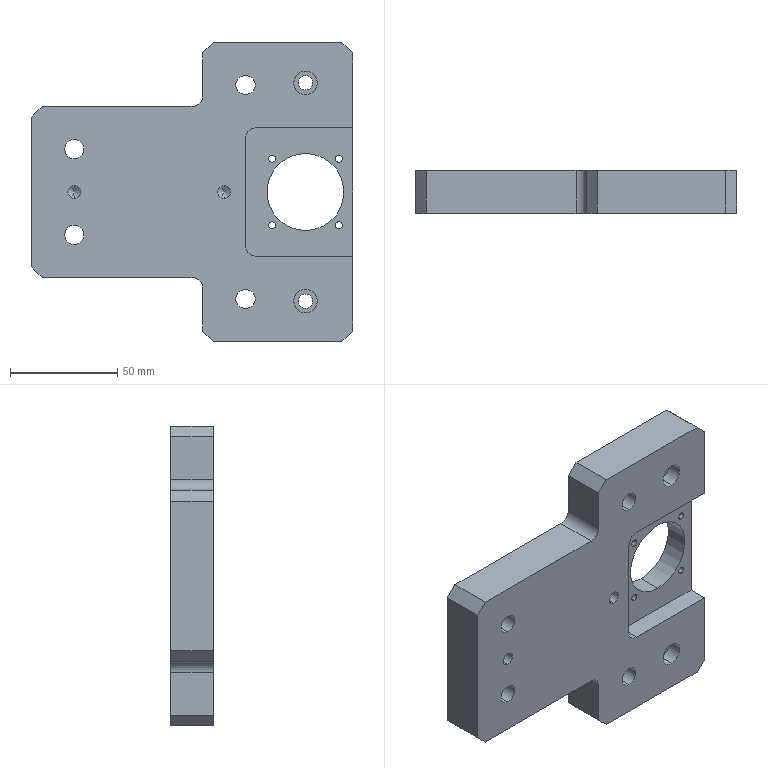Part | SolidWorks | features HoleWzd 7, Chamfer 2, Cut 2, Fillet 2, ICE 2, Extrusion 1 | 1 solid | 98 faces | box 150 x 20 x 140 mm | volume 269906 mm3 | cylinder 56 | plane 28 | cone 14 | commonest cylinder face diameters 3.3 x10 5 x8 9 x8 15 x8 6 x4 6.6 x4